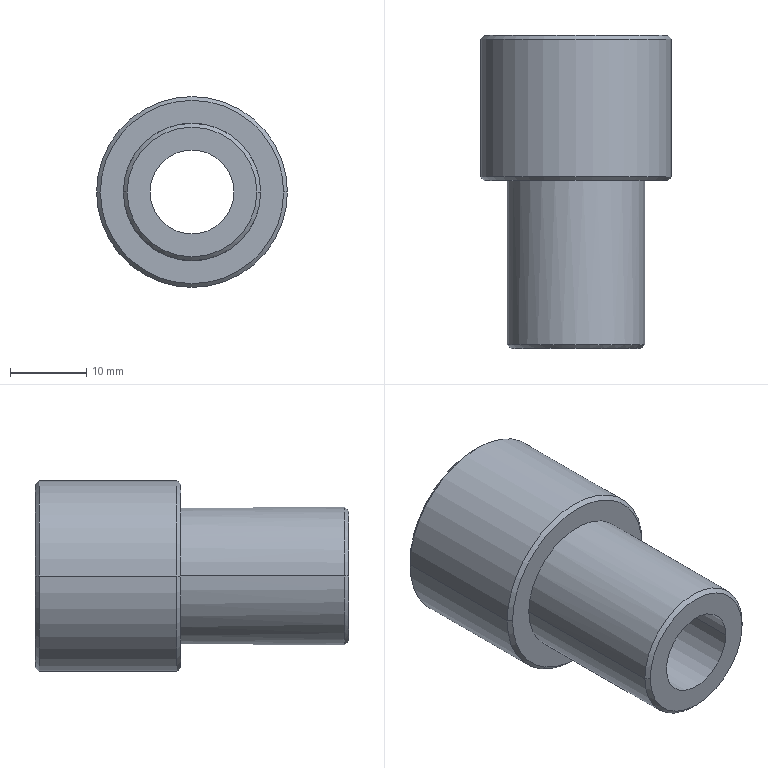Part | Creo | 1 solid | 20 faces | box 25 x 41 x 25 mm | volume 8763 mm3 | cylinder 8 | cone 8 | plane 4 | commonest cylinder face diameters 18 x4 11 x2 25 x2
STEP:
#1=CARTESIAN_POINT('',(-17.576,325.995,-174.076));
#2=VERTEX_POINT('',#1);
#3=CARTESIAN_POINT('',(-17.576,352.995,-174.076));
#4=VERTEX_POINT('',#3);
#5=CARTESIAN_POINT('',(-17.576,325.995,-174.076));
#6=DIRECTION('',(0.,1.,0.));
#7=VECTOR('',#6,27.);
#8=LINE('',#5,#7);
#9=EDGE_CURVE('',#2,#4,#8,.T.);
#10=ORIENTED_EDGE('',*,*,#9,.F.);
#11=CARTESIAN_POINT('',(-28.576,325.995,-174.076));
#12=VERTEX_POINT('',#11);
#13=CARTESIAN_POINT('',(-23.076,325.995,-174.076));
#14=DIRECTION('',(0.,1.,0.));
#15=DIRECTION('',(1.,0.,0.));
#16=AXIS2_PLACEMENT_3D('',#13,#14,#15);
#17=CIRCLE('',#16,5.5);
#18=EDGE_CURVE('',#2,#12,#17,.T.);
#19=ORIENTED_EDGE('',*,*,#18,.T.);
#20=CARTESIAN_POINT('',(-28.576,352.995,-174.076));
#21=VERTEX_POINT('',#20);
#22=CARTESIAN_POINT('',(-28.576,352.995,-174.076));
#23=DIRECTION('',(0.,-1.,0.));
#24=VECTOR('',#23,27.);
#25=LINE('',#22,#24);
#26=EDGE_CURVE('',#21,#12,#25,.T.);
#27=ORIENTED_EDGE('',*,*,#26,.F.);
#28=CARTESIAN_POINT('',(-23.076,352.995,-174.076));
#29=DIRECTION('',(0.,-1.,0.));
#30=DIRECTION('',(-1.,0.,0.));
#31=AXIS2_PLACEMENT_3D('',#28,#29,#30);
#32=CIRCLE('',#31,5.5);
#33=EDGE_CURVE('',#21,#4,#32,.T.);
#34=ORIENTED_EDGE('',*,*,#33,.T.);
#35=EDGE_LOOP('',(#10,#19,#27,#34));
#36=FACE_OUTER_BOUND('',#35,.F.);
#37=CARTESIAN_POINT('',(-23.076,343.995,-174.076));
#38=DIRECTION('',(0.,1.,0.));
#39=DIRECTION('',(-1.,0.,0.));
#40=AXIS2_PLACEMENT_3D('',#37,#38,#39);
#41=CYLINDRICAL_SURFACE('',#40,5.5);
#42=ADVANCED_FACE('',(#36),#41,.F.);
#43=ORIENTED_EDGE('',*,*,#26,.T.);
#44=CARTESIAN_POINT('',(-23.076,325.995,-174.076));
#45=DIRECTION('',(0.,1.,0.));
#46=DIRECTION('',(-1.,0.,0.));
#47=AXIS2_PLACEMENT_3D('',#44,#45,#46);
#48=CIRCLE('',#47,5.5);
#49=EDGE_CURVE('',#12,#2,#48,.T.);
#50=ORIENTED_EDGE('',*,*,#49,.T.);
#51=ORIENTED_EDGE('',*,*,#9,.T.);
#52=CARTESIAN_POINT('',(-23.076,352.995,-174.076));
#53=DIRECTION('',(0.,-1.,0.));
#54=DIRECTION('',(1.,0.,0.));
#55=AXIS2_PLACEMENT_3D('',#52,#53,#54);
#56=CIRCLE('',#55,5.5);
#57=EDGE_CURVE('',#4,#21,#56,.T.);
#58=ORIENTED_EDGE('',*,*,#57,.T.);
#59=EDGE_LOOP('',(#43,#50,#51,#58));
#60=FACE_OUTER_BOUND('',#59,.F.);
#61=CARTESIAN_POINT('',(-23.076,343.995,-174.076));
#62=DIRECTION('',(0.,1.,0.));
#63=DIRECTION('',(-1.,0.,0.));
#64=AXIS2_PLACEMENT_3D('',#61,#62,#63);
#65=CYLINDRICAL_SURFACE('',#64,5.5);
#66=ADVANCED_FACE('',(#60),#65,.F.);
#67=CARTESIAN_POINT('',(-31.576,325.995,-174.076));
#68=VERTEX_POINT('',#67);
#69=CARTESIAN_POINT('',(-23.076,325.995,-182.576));
#70=VERTEX_POINT('',#69);
#71=CARTESIAN_POINT('',(-23.076,325.995,-174.076));
#72=DIRECTION('',(0.,-1.,0.));
#73=DIRECTION('',(-1.,0.,0.));
#74=AXIS2_PLACEMENT_3D('',#71,#72,#73);
#75=CIRCLE('',#74,8.5);
#76=EDGE_CURVE('',#68,#70,#75,.T.);
#77=ORIENTED_EDGE('',*,*,#76,.F.);
#78=CARTESIAN_POINT('',(-23.076,325.995,-165.576));
#79=VERTEX_POINT('',#78);
#80=CARTESIAN_POINT('',(-23.076,325.995,-174.076));
#81=DIRECTION('',(0.,-1.,0.));
#82=DIRECTION('',(0.,0.,1.));
#83=AXIS2_PLACEMENT_3D('',#80,#81,#82);
#84=CIRCLE('',#83,8.5);
#85=EDGE_CURVE('',#79,#68,#84,.T.);
#86=ORIENTED_EDGE('',*,*,#85,.F.);
#87=CARTESIAN_POINT('',(-14.576,325.995,-174.076));
#88=VERTEX_POINT('',#87);
#89=CARTESIAN_POINT('',(-23.076,325.995,-174.076));
#90=DIRECTION('',(0.,-1.,0.));
#91=DIRECTION('',(1.,0.,0.));
#92=AXIS2_PLACEMENT_3D('',#89,#90,#91);
#93=CIRCLE('',#92,8.5);
#94=EDGE_CURVE('',#88,#79,#93,.T.);
#95=ORIENTED_EDGE('',*,*,#94,.F.);
#96=CARTESIAN_POINT('',(-23.076,325.995,-174.076));
#97=DIRECTION('',(0.,-1.,0.));
#98=DIRECTION('',(0.,0.,-1.));
#99=AXIS2_PLACEMENT_3D('',#96,#97,#98);
#100=CIRCLE('',#99,8.5);
#101=EDGE_CURVE('',#70,#88,#100,.T.);
#102=ORIENTED_EDGE('',*,*,#101,.F.);
#103=EDGE_LOOP('',(#77,#86,#95,#102));
#104=FACE_OUTER_BOUND('',#103,.F.);
#105=ORIENTED_EDGE('',*,*,#18,.F.);
#106=ORIENTED_EDGE('',*,*,#49,.F.);
#107=EDGE_LOOP('',(#105,#106));
#108=FACE_BOUND('',#107,.F.);
#109=CARTESIAN_POINT('',(16.924,325.995,-304.076));
#110=DIRECTION('',(0.,-1.,0.));
#111=DIRECTION('',(-1.,0.,0.));
#112=AXIS2_PLACEMENT_3D('',#109,#110,#111);
#113=PLANE('',#112);
#114=ADVANCED_FACE('',(#104,#108),#113,.T.);
#115=CARTESIAN_POINT('',(-32.076,326.495,-174.076));
#116=VERTEX_POINT('',#115);
#117=CARTESIAN_POINT('',(-31.576,325.995,-174.076));
#118=DIRECTION('',(-0.7071,0.7071,-0.000000008));
#119=VECTOR('',#118,0.7071);
#120=LINE('',#117,#119);
#121=EDGE_CURVE('',#68,#116,#120,.T.);
#122=ORIENTED_EDGE('',*,*,#121,.F.);
#123=ORIENTED_EDGE('',*,*,#76,.T.);
#124=ORIENTED_EDGE('',*,*,#101,.T.);
#125=CARTESIAN_POINT('',(-14.076,326.495,-174.076));
#126=VERTEX_POINT('',#125);
#127=CARTESIAN_POINT('',(-14.076,326.495,-174.076));
#128=DIRECTION('',(-0.7071,-0.7071,-0.000000008));
#129=VECTOR('',#128,0.7071);
#130=LINE('',#127,#129);
#131=EDGE_CURVE('',#126,#88,#130,.T.);
#132=ORIENTED_EDGE('',*,*,#131,.F.);
#133=CARTESIAN_POINT('',(-23.076,326.495,-183.076));
#134=VERTEX_POINT('',#133);
#135=CARTESIAN_POINT('',(-23.076,326.495,-174.076));
#136=DIRECTION('',(0.,-1.,0.));
#137=DIRECTION('',(0.,0.,-1.));
#138=AXIS2_PLACEMENT_3D('',#135,#136,#137);
#139=CIRCLE('',#138,9.);
#140=EDGE_CURVE('',#134,#126,#139,.T.);
#141=ORIENTED_EDGE('',*,*,#140,.F.);
#142=CARTESIAN_POINT('',(-23.076,326.495,-174.076));
#143=DIRECTION('',(0.,-1.,0.));
#144=DIRECTION('',(-1.,0.,0.));
#145=AXIS2_PLACEMENT_3D('',#142,#143,#144);
#146=CIRCLE('',#145,9.);
#147=EDGE_CURVE('',#116,#134,#146,.T.);
#148=ORIENTED_EDGE('',*,*,#147,.F.);
#149=EDGE_LOOP('',(#122,#123,#124,#132,#141,#148));
#150=FACE_OUTER_BOUND('',#149,.F.);
#151=CARTESIAN_POINT('',(-23.076,326.245,-174.076));
#152=DIRECTION('',(0.,1.,0.));
#153=DIRECTION('',(0.,0.,1.));
#154=AXIS2_PLACEMENT_3D('',#151,#152,#153);
#155=CONICAL_SURFACE('',#154,8.75,45.);
#156=ADVANCED_FACE('',(#150),#155,.T.);
#157=ORIENTED_EDGE('',*,*,#131,.T.);
#158=ORIENTED_EDGE('',*,*,#94,.T.);
#159=ORIENTED_EDGE('',*,*,#85,.T.);
#160=ORIENTED_EDGE('',*,*,#121,.T.);
#161=CARTESIAN_POINT('',(-23.076,326.495,-165.076));
#162=VERTEX_POINT('',#161);
#163=CARTESIAN_POINT('',(-23.076,326.495,-174.076));
#164=DIRECTION('',(0.,-1.,0.));
#165=DIRECTION('',(0.,0.,1.));
#166=AXIS2_PLACEMENT_3D('',#163,#164,#165);
#167=CIRCLE('',#166,9.);
#168=EDGE_CURVE('',#162,#116,#167,.T.);
#169=ORIENTED_EDGE('',*,*,#168,.F.);
#170=CARTESIAN_POINT('',(-23.076,326.495,-174.076));
#171=DIRECTION('',(0.,-1.,0.));
#172=DIRECTION('',(1.,0.,0.));
#173=AXIS2_PLACEMENT_3D('',#170,#171,#172);
#174=CIRCLE('',#173,9.);
#175=EDGE_CURVE('',#126,#162,#174,.T.);
#176=ORIENTED_EDGE('',*,*,#175,.F.);
#177=EDGE_LOOP('',(#157,#158,#159,#160,#169,#176));
#178=FACE_OUTER_BOUND('',#177,.F.);
#179=CARTESIAN_POINT('',(-23.076,326.245,-174.076));
#180=DIRECTION('',(0.,1.,0.));
#181=DIRECTION('',(0.,0.,1.));
#182=AXIS2_PLACEMENT_3D('',#179,#180,#181);
#183=CONICAL_SURFACE('',#182,8.75,45.);
#184=ADVANCED_FACE('',(#178),#183,.T.);
#185=CARTESIAN_POINT('',(-14.076,347.995,-174.076));
#186=VERTEX_POINT('',#185);
#187=CARTESIAN_POINT('',(-14.076,326.495,-174.076));
#188=DIRECTION('',(0.,1.,0.000000001));
#189=VECTOR('',#188,21.5);
#190=LINE('',#187,#189);
#191=EDGE_CURVE('',#126,#186,#190,.T.);
#192=ORIENTED_EDGE('',*,*,#191,.F.);
#193=ORIENTED_EDGE('',*,*,#175,.T.);
#194=ORIENTED_EDGE('',*,*,#168,.T.);
#195=CARTESIAN_POINT('',(-32.076,347.995,-174.076));
#196=VERTEX_POINT('',#195);
#197=CARTESIAN_POINT('',(-32.076,347.995,-174.076));
#198=DIRECTION('',(0.,-1.,0.000000001));
#199=VECTOR('',#198,21.5);
#200=LINE('',#197,#199);
#201=EDGE_CURVE('',#196,#116,#200,.T.);
#202=ORIENTED_EDGE('',*,*,#201,.F.);
#203=CARTESIAN_POINT('',(-23.076,347.995,-174.076));
#204=DIRECTION('',(0.,1.,0.));
#205=DIRECTION('',(-1.,0.,0.));
#206=AXIS2_PLACEMENT_3D('',#203,#204,#205);
#207=CIRCLE('',#206,9.);
#208=EDGE_CURVE('',#196,#186,#207,.T.);
#209=ORIENTED_EDGE('',*,*,#208,.T.);
#210=EDGE_LOOP('',(#192,#193,#194,#202,#209));
#211=FACE_OUTER_BOUND('',#210,.F.);
#212=CARTESIAN_POINT('',(-23.076,319.995,-174.076));
#213=DIRECTION('',(0.,-1.,0.));
#214=DIRECTION('',(-1.,0.,0.));
#215=AXIS2_PLACEMENT_3D('',#212,#213,#214);
#216=CYLINDRICAL_SURFACE('',#215,9.);
#217=ADVANCED_FACE('',(#211),#216,.T.);
#218=ORIENTED_EDGE('',*,*,#201,.T.);
#219=ORIENTED_EDGE('',*,*,#147,.T.);
#220=ORIENTED_EDGE('',*,*,#140,.T.);
#221=ORIENTED_EDGE('',*,*,#191,.T.);
#222=CARTESIAN_POINT('',(-23.076,347.995,-174.076));
#223=DIRECTION('',(0.,1.,0.));
#224=DIRECTION('',(1.,0.,0.));
#225=AXIS2_PLACEMENT_3D('',#222,#223,#224);
#226=CIRCLE('',#225,9.);
#227=EDGE_CURVE('',#186,#196,#226,.T.);
#228=ORIENTED_EDGE('',*,*,#227,.T.);
#229=EDGE_LOOP('',(#218,#219,#220,#221,#228));
#230=FACE_OUTER_BOUND('',#229,.F.);
#231=CARTESIAN_POINT('',(-23.076,319.995,-174.076));
#232=DIRECTION('',(0.,-1.,0.));
#233=DIRECTION('',(-1.,0.,0.));
#234=AXIS2_PLACEMENT_3D('',#231,#232,#233);
#235=CYLINDRICAL_SURFACE('',#234,9.);
#236=ADVANCED_FACE('',(#230),#235,.T.);
#237=CARTESIAN_POINT('',(-35.076,347.995,-174.076));
#238=VERTEX_POINT('',#237);
#239=CARTESIAN_POINT('',(-23.076,347.995,-186.076));
#240=VERTEX_POINT('',#239);
#241=CARTESIAN_POINT('',(-23.076,347.995,-174.076));
#242=DIRECTION('',(0.,-1.,0.));
#243=DIRECTION('',(-1.,0.,0.));
#244=AXIS2_PLACEMENT_3D('',#241,#242,#243);
#245=CIRCLE('',#244,12.);
#246=EDGE_CURVE('',#238,#240,#245,.T.);
#247=ORIENTED_EDGE('',*,*,#246,.F.);
#248=CARTESIAN_POINT('',(-23.076,347.995,-162.076));
#249=VERTEX_POINT('',#248);
#250=CARTESIAN_POINT('',(-23.076,347.995,-174.076));
#251=DIRECTION('',(0.,-1.,0.));
#252=DIRECTION('',(0.,0.,1.));
#253=AXIS2_PLACEMENT_3D('',#250,#251,#252);
#254=CIRCLE('',#253,12.);
#255=EDGE_CURVE('',#249,#238,#254,.T.);
#256=ORIENTED_EDGE('',*,*,#255,.F.);
#257=CARTESIAN_POINT('',(-11.076,347.995,-174.076));
#258=VERTEX_POINT('',#257);
#259=CARTESIAN_POINT('',(-23.076,347.995,-174.076));
#260=DIRECTION('',(0.,-1.,0.));
#261=DIRECTION('',(1.,0.,0.));
#262=AXIS2_PLACEMENT_3D('',#259,#260,#261);
#263=CIRCLE('',#262,12.);
#264=EDGE_CURVE('',#258,#249,#263,.T.);
#265=ORIENTED_EDGE('',*,*,#264,.F.);
#266=CARTESIAN_POINT('',(-23.076,347.995,-174.076));
#267=DIRECTION('',(0.,-1.,0.));
#268=DIRECTION('',(0.,0.,-1.));
#269=AXIS2_PLACEMENT_3D('',#266,#267,#268);
#270=CIRCLE('',#269,12.);
#271=EDGE_CURVE('',#240,#258,#270,.T.);
#272=ORIENTED_EDGE('',*,*,#271,.F.);
#273=EDGE_LOOP('',(#247,#256,#265,#272));
#274=FACE_OUTER_BOUND('',#273,.F.);
#275=ORIENTED_EDGE('',*,*,#227,.F.);
#276=ORIENTED_EDGE('',*,*,#208,.F.);
#277=EDGE_LOOP('',(#275,#276));
#278=FACE_BOUND('',#277,.F.);
#279=CARTESIAN_POINT('',(16.924,347.995,-304.076));
#280=DIRECTION('',(0.,-1.,0.));
#281=DIRECTION('',(-1.,0.,0.));
#282=AXIS2_PLACEMENT_3D('',#279,#280,#281);
#283=PLANE('',#282);
#284=ADVANCED_FACE('',(#274,#278),#283,.T.);
#285=CARTESIAN_POINT('',(-10.576,348.495,-174.076));
#286=VERTEX_POINT('',#285);
#287=CARTESIAN_POINT('',(-11.076,347.995,-174.076));
#288=DIRECTION('',(0.7071,0.7071,-0.000000007));
#289=VECTOR('',#288,0.7071);
#290=LINE('',#287,#289);
#291=EDGE_CURVE('',#258,#286,#290,.T.);
#292=ORIENTED_EDGE('',*,*,#291,.T.);
#293=CARTESIAN_POINT('',(-23.076,348.495,-186.576));
#294=VERTEX_POINT('',#293);
#295=CARTESIAN_POINT('',(-23.076,348.495,-174.076));
#296=DIRECTION('',(0.,-1.,0.));
#297=DIRECTION('',(0.,0.,-1.));
#298=AXIS2_PLACEMENT_3D('',#295,#296,#297);
#299=CIRCLE('',#298,12.5);
#300=EDGE_CURVE('',#294,#286,#299,.T.);
#301=ORIENTED_EDGE('',*,*,#300,.F.);
#302=CARTESIAN_POINT('',(-35.576,348.495,-174.076));
#303=VERTEX_POINT('',#302);
#304=CARTESIAN_POINT('',(-23.076,348.495,-174.076));
#305=DIRECTION('',(0.,-1.,0.));
#306=DIRECTION('',(-1.,0.,0.));
#307=AXIS2_PLACEMENT_3D('',#304,#305,#306);
#308=CIRCLE('',#307,12.5);
#309=EDGE_CURVE('',#303,#294,#308,.T.);
#310=ORIENTED_EDGE('',*,*,#309,.F.);
#311=CARTESIAN_POINT('',(-35.576,348.495,-174.076));
#312=DIRECTION('',(0.7071,-0.7071,-0.000000007));
#313=VECTOR('',#312,0.7071);
#314=LINE('',#311,#313);
#315=EDGE_CURVE('',#303,#238,#314,.T.);
#316=ORIENTED_EDGE('',*,*,#315,.T.);
#317=ORIENTED_EDGE('',*,*,#246,.T.);
#318=ORIENTED_EDGE('',*,*,#271,.T.);
#319=EDGE_LOOP('',(#292,#301,#310,#316,#317,#318));
#320=FACE_OUTER_BOUND('',#319,.F.);
#321=CARTESIAN_POINT('',(-23.076,348.245,-174.076));
#322=DIRECTION('',(0.,1.,0.));
#323=DIRECTION('',(0.,0.,1.));
#324=AXIS2_PLACEMENT_3D('',#321,#322,#323);
#325=CONICAL_SURFACE('',#324,12.25,45.);
#326=ADVANCED_FACE('',(#320),#325,.T.);
#327=ORIENTED_EDGE('',*,*,#315,.F.);
#328=CARTESIAN_POINT('',(-23.076,348.495,-161.576));
#329=VERTEX_POINT('',#328);
#330=CARTESIAN_POINT('',(-23.076,348.495,-174.076));
#331=DIRECTION('',(0.,-1.,0.));
#332=DIRECTION('',(0.,0.,1.));
#333=AXIS2_PLACEMENT_3D('',#330,#331,#332);
#334=CIRCLE('',#333,12.5);
#335=EDGE_CURVE('',#329,#303,#334,.T.);
#336=ORIENTED_EDGE('',*,*,#335,.F.);
#337=CARTESIAN_POINT('',(-23.076,348.495,-174.076));
#338=DIRECTION('',(0.,-1.,0.));
#339=DIRECTION('',(1.,0.,0.));
#340=AXIS2_PLACEMENT_3D('',#337,#338,#339);
#341=CIRCLE('',#340,12.5);
#342=EDGE_CURVE('',#286,#329,#341,.T.);
#343=ORIENTED_EDGE('',*,*,#342,.F.);
#344=ORIENTED_EDGE('',*,*,#291,.F.);
#345=ORIENTED_EDGE('',*,*,#264,.T.);
#346=ORIENTED_EDGE('',*,*,#255,.T.);
#347=EDGE_LOOP('',(#327,#336,#343,#344,#345,#346));
#348=FACE_OUTER_BOUND('',#347,.F.);
#349=CARTESIAN_POINT('',(-23.076,348.245,-174.076));
#350=DIRECTION('',(0.,1.,0.));
#351=DIRECTION('',(0.,0.,1.));
#352=AXIS2_PLACEMENT_3D('',#349,#350,#351);
#353=CONICAL_SURFACE('',#352,12.25,45.);
#354=ADVANCED_FACE('',(#348),#353,.T.);
#355=CARTESIAN_POINT('',(-35.576,366.495,-174.076));
#356=VERTEX_POINT('',#355);
#357=CARTESIAN_POINT('',(-35.576,366.495,-174.076));
#358=DIRECTION('',(0.,-1.,0.));
#359=VECTOR('',#358,18.);
#360=LINE('',#357,#359);
#361=EDGE_CURVE('',#356,#303,#360,.T.);
#362=ORIENTED_EDGE('',*,*,#361,.F.);
#363=CARTESIAN_POINT('',(-23.076,366.495,-161.576));
#364=VERTEX_POINT('',#363);
#365=CARTESIAN_POINT('',(-23.076,366.495,-174.076));
#366=DIRECTION('',(0.,1.,0.));
#367=DIRECTION('',(-1.,0.,0.));
#368=AXIS2_PLACEMENT_3D('',#365,#366,#367);
#369=CIRCLE('',#368,12.5);
#370=EDGE_CURVE('',#356,#364,#369,.T.);
#371=ORIENTED_EDGE('',*,*,#370,.T.);
#372=CARTESIAN_POINT('',(-10.576,366.495,-174.076));
#373=VERTEX_POINT('',#372);
#374=CARTESIAN_POINT('',(-23.076,366.495,-174.076));
#375=DIRECTION('',(0.,1.,0.));
#376=DIRECTION('',(0.,0.,1.));
#377=AXIS2_PLACEMENT_3D('',#374,#375,#376);
#378=CIRCLE('',#377,12.5);
#379=EDGE_CURVE('',#364,#373,#378,.T.);
#380=ORIENTED_EDGE('',*,*,#379,.T.);
#381=CARTESIAN_POINT('',(-10.576,348.495,-174.076));
#382=DIRECTION('',(0.,1.,0.));
#383=VECTOR('',#382,18.);
#384=LINE('',#381,#383);
#385=EDGE_CURVE('',#286,#373,#384,.T.);
#386=ORIENTED_EDGE('',*,*,#385,.F.);
#387=ORIENTED_EDGE('',*,*,#342,.T.);
#388=ORIENTED_EDGE('',*,*,#335,.T.);
#389=EDGE_LOOP('',(#362,#371,#380,#386,#387,#388));
#390=FACE_OUTER_BOUND('',#389,.F.);
#391=CARTESIAN_POINT('',(-23.076,328.995,-174.076));
#392=DIRECTION('',(0.,-1.,0.));
#393=DIRECTION('',(-1.,0.,0.));
#394=AXIS2_PLACEMENT_3D('',#391,#392,#393);
#395=CYLINDRICAL_SURFACE('',#394,12.5);
#396=ADVANCED_FACE('',(#390),#395,.T.);
#397=ORIENTED_EDGE('',*,*,#385,.T.);
#398=CARTESIAN_POINT('',(-23.076,366.495,-186.576));
#399=VERTEX_POINT('',#398);
#400=CARTESIAN_POINT('',(-23.076,366.495,-174.076));
#401=DIRECTION('',(0.,1.,0.));
#402=DIRECTION('',(1.,0.,0.));
#403=AXIS2_PLACEMENT_3D('',#400,#401,#402);
#404=CIRCLE('',#403,12.5);
#405=EDGE_CURVE('',#373,#399,#404,.T.);
#406=ORIENTED_EDGE('',*,*,#405,.T.);
#407=CARTESIAN_POINT('',(-23.076,366.495,-174.076));
#408=DIRECTION('',(0.,1.,0.));
#409=DIRECTION('',(0.,0.,-1.));
#410=AXIS2_PLACEMENT_3D('',#407,#408,#409);
#411=CIRCLE('',#410,12.5);
#412=EDGE_CURVE('',#399,#356,#411,.T.);
#413=ORIENTED_EDGE('',*,*,#412,.T.);
#414=ORIENTED_EDGE('',*,*,#361,.T.);
#415=ORIENTED_EDGE('',*,*,#309,.T.);
#416=ORIENTED_EDGE('',*,*,#300,.T.);
#417=EDGE_LOOP('',(#397,#406,#413,#414,#415,#416));
#418=FACE_OUTER_BOUND('',#417,.F.);
#419=CARTESIAN_POINT('',(-23.076,328.995,-174.076));
#420=DIRECTION('',(0.,-1.,0.));
#421=DIRECTION('',(-1.,0.,0.));
#422=AXIS2_PLACEMENT_3D('',#419,#420,#421);
#423=CYLINDRICAL_SURFACE('',#422,12.5);
#424=ADVANCED_FACE('',(#418),#423,.T.);
#425=CARTESIAN_POINT('',(-11.076,366.995,-174.076));
#426=VERTEX_POINT('',#425);
#427=CARTESIAN_POINT('',(-10.576,366.495,-174.076));
#428=DIRECTION('',(-0.7071,0.7071,0.000000011));
#429=VECTOR('',#428,0.7071);
#430=LINE('',#427,#429);
#431=EDGE_CURVE('',#373,#426,#430,.T.);
#432=ORIENTED_EDGE('',*,*,#431,.T.);
#433=CARTESIAN_POINT('',(-23.076,366.995,-186.076));
#434=VERTEX_POINT('',#433);
#435=CARTESIAN_POINT('',(-23.076,366.995,-174.076));
#436=DIRECTION('',(0.,1.,0.));
#437=DIRECTION('',(1.,0.,0.));
#438=AXIS2_PLACEMENT_3D('',#435,#436,#437);
#439=CIRCLE('',#438,12.);
#440=EDGE_CURVE('',#426,#434,#439,.T.);
#441=ORIENTED_EDGE('',*,*,#440,.T.);
#442=CARTESIAN_POINT('',(-35.076,366.995,-174.076));
#443=VERTEX_POINT('',#442);
#444=CARTESIAN_POINT('',(-23.076,366.995,-174.076));
#445=DIRECTION('',(0.,1.,0.));
#446=DIRECTION('',(0.,0.,-1.));
#447=AXIS2_PLACEMENT_3D('',#444,#445,#446);
#448=CIRCLE('',#447,12.);
#449=EDGE_CURVE('',#434,#443,#448,.T.);
#450=ORIENTED_EDGE('',*,*,#449,.T.);
#451=CARTESIAN_POINT('',(-35.076,366.995,-174.076));
#452=DIRECTION('',(-0.7071,-0.7071,0.000000011));
#453=VECTOR('',#452,0.7071);
#454=LINE('',#451,#453);
#455=EDGE_CURVE('',#443,#356,#454,.T.);
#456=ORIENTED_EDGE('',*,*,#455,.T.);
#457=ORIENTED_EDGE('',*,*,#412,.F.);
#458=ORIENTED_EDGE('',*,*,#405,.F.);
#459=EDGE_LOOP('',(#432,#441,#450,#456,#457,#458));
#460=FACE_OUTER_BOUND('',#459,.F.);
#461=CARTESIAN_POINT('',(-23.076,366.745,-174.076));
#462=DIRECTION('',(0.,-1.,0.));
#463=DIRECTION('',(0.,0.,1.));
#464=AXIS2_PLACEMENT_3D('',#461,#462,#463);
#465=CONICAL_SURFACE('',#464,12.25,45.);
#466=ADVANCED_FACE('',(#460),#465,.T.);
#467=ORIENTED_EDGE('',*,*,#455,.F.);
#468=CARTESIAN_POINT('',(-23.076,366.995,-162.076));
#469=VERTEX_POINT('',#468);
#470=CARTESIAN_POINT('',(-23.076,366.995,-174.076));
#471=DIRECTION('',(0.,1.,0.));
#472=DIRECTION('',(-1.,0.,0.));
#473=AXIS2_PLACEMENT_3D('',#470,#471,#472);
#474=CIRCLE('',#473,12.);
#475=EDGE_CURVE('',#443,#469,#474,.T.);
#476=ORIENTED_EDGE('',*,*,#475,.T.);
#477=CARTESIAN_POINT('',(-23.076,366.995,-174.076));
#478=DIRECTION('',(0.,1.,0.));
#479=DIRECTION('',(0.,0.,1.));
#480=AXIS2_PLACEMENT_3D('',#477,#478,#479);
#481=CIRCLE('',#480,12.);
#482=EDGE_CURVE('',#469,#426,#481,.T.);
#483=ORIENTED_EDGE('',*,*,#482,.T.);
#484=ORIENTED_EDGE('',*,*,#431,.F.);
#485=ORIENTED_EDGE('',*,*,#379,.F.);
#486=ORIENTED_EDGE('',*,*,#370,.F.);
#487=EDGE_LOOP('',(#467,#476,#483,#484,#485,#486));
#488=FACE_OUTER_BOUND('',#487,.F.);
#489=CARTESIAN_POINT('',(-23.076,366.745,-174.076));
#490=DIRECTION('',(0.,-1.,0.));
#491=DIRECTION('',(0.,0.,1.));
#492=AXIS2_PLACEMENT_3D('',#489,#490,#491);
#493=CONICAL_SURFACE('',#492,12.25,45.);
#494=ADVANCED_FACE('',(#488),#493,.T.);
#495=ORIENTED_EDGE('',*,*,#440,.F.);
#496=ORIENTED_EDGE('',*,*,#482,.F.);
#497=ORIENTED_EDGE('',*,*,#475,.F.);
#498=ORIENTED_EDGE('',*,*,#449,.F.);
#499=EDGE_LOOP('',(#495,#496,#497,#498));
#500=FACE_OUTER_BOUND('',#499,.F.);
#501=CARTESIAN_POINT('',(-32.576,366.995,-174.076));
#502=VERTEX_POINT('',#501);
#503=CARTESIAN_POINT('',(-23.076,366.995,-183.576));
#504=VERTEX_POINT('',#503);
#505=CARTESIAN_POINT('',(-23.076,366.995,-174.076));
#506=DIRECTION('',(0.,-1.,0.));
#507=DIRECTION('',(-1.,0.,0.));
#508=AXIS2_PLACEMENT_3D('',#505,#506,#507);
#509=CIRCLE('',#508,9.5);
#510=EDGE_CURVE('',#502,#504,#509,.T.);
#511=ORIENTED_EDGE('',*,*,#510,.F.);
#512=CARTESIAN_POINT('',(-23.076,366.995,-164.576));
#513=VERTEX_POINT('',#512);
#514=CARTESIAN_POINT('',(-23.076,366.995,-174.076));
#515=DIRECTION('',(0.,-1.,0.));
#516=DIRECTION('',(0.,0.,1.));
#517=AXIS2_PLACEMENT_3D('',#514,#515,#516);
#518=CIRCLE('',#517,9.5);
#519=EDGE_CURVE('',#513,#502,#518,.T.);
#520=ORIENTED_EDGE('',*,*,#519,.F.);
#521=CARTESIAN_POINT('',(-13.576,366.995,-174.076));
#522=VERTEX_POINT('',#521);
#523=CARTESIAN_POINT('',(-23.076,366.995,-174.076));
#524=DIRECTION('',(0.,-1.,0.));
#525=DIRECTION('',(1.,0.,0.));
#526=AXIS2_PLACEMENT_3D('',#523,#524,#525);
#527=CIRCLE('',#526,9.5);
#528=EDGE_CURVE('',#522,#513,#527,.T.);
#529=ORIENTED_EDGE('',*,*,#528,.F.);
#530=CARTESIAN_POINT('',(-23.076,366.995,-174.076));
#531=DIRECTION('',(0.,-1.,0.));
#532=DIRECTION('',(0.,0.,-1.));
#533=AXIS2_PLACEMENT_3D('',#530,#531,#532);
#534=CIRCLE('',#533,9.5);
#535=EDGE_CURVE('',#504,#522,#534,.T.);
#536=ORIENTED_EDGE('',*,*,#535,.F.);
#537=EDGE_LOOP('',(#511,#520,#529,#536));
#538=FACE_BOUND('',#537,.F.);
#539=CARTESIAN_POINT('',(16.924,366.995,-304.076));
#540=DIRECTION('',(0.,-1.,0.));
#541=DIRECTION('',(-1.,0.,0.));
#542=AXIS2_PLACEMENT_3D('',#539,#540,#541);
#543=PLANE('',#542);
#544=ADVANCED_FACE('',(#500,#538),#543,.F.);
#545=CARTESIAN_POINT('',(-32.076,366.495,-174.076));
#546=VERTEX_POINT('',#545);
#547=CARTESIAN_POINT('',(-32.576,366.995,-174.076));
#548=DIRECTION('',(0.7071,-0.7071,-0.000000021));
#549=VECTOR('',#548,0.7071);
#550=LINE('',#547,#549);
#551=EDGE_CURVE('',#502,#546,#550,.T.);
#552=ORIENTED_EDGE('',*,*,#551,.F.);
#553=ORIENTED_EDGE('',*,*,#510,.T.);
#554=ORIENTED_EDGE('',*,*,#535,.T.);
#555=CARTESIAN_POINT('',(-14.076,366.495,-174.076));
#556=VERTEX_POINT('',#555);
#557=CARTESIAN_POINT('',(-14.076,366.495,-174.076));
#558=DIRECTION('',(0.7071,0.7071,-0.000000021));
#559=VECTOR('',#558,0.7071);
#560=LINE('',#557,#559);
#561=EDGE_CURVE('',#556,#522,#560,.T.);
#562=ORIENTED_EDGE('',*,*,#561,.F.);
#563=CARTESIAN_POINT('',(-23.076,366.495,-183.076));
#564=VERTEX_POINT('',#563);
#565=CARTESIAN_POINT('',(-23.076,366.495,-174.076));
#566=DIRECTION('',(0.,-1.,0.));
#567=DIRECTION('',(0.,0.,-1.));
#568=AXIS2_PLACEMENT_3D('',#565,#566,#567);
#569=CIRCLE('',#568,9.);
#570=EDGE_CURVE('',#564,#556,#569,.T.);
#571=ORIENTED_EDGE('',*,*,#570,.F.);
#572=CARTESIAN_POINT('',(-23.076,366.495,-174.076));
#573=DIRECTION('',(0.,-1.,0.));
#574=DIRECTION('',(-1.,0.,0.));
#575=AXIS2_PLACEMENT_3D('',#572,#573,#574);
#576=CIRCLE('',#575,9.);
#577=EDGE_CURVE('',#546,#564,#576,.T.);
#578=ORIENTED_EDGE('',*,*,#577,.F.);
#579=EDGE_LOOP('',(#552,#553,#554,#562,#571,#578));
#580=FACE_OUTER_BOUND('',#579,.F.);
#581=CARTESIAN_POINT('',(-23.076,366.745,-174.076));
#582=DIRECTION('',(0.,1.,0.));
#583=DIRECTION('',(0.,0.,1.));
#584=AXIS2_PLACEMENT_3D('',#581,#582,#583);
#585=CONICAL_SURFACE('',#584,9.25,45.);
#586=ADVANCED_FACE('',(#580),#585,.F.);
#587=ORIENTED_EDGE('',*,*,#561,.T.);
#588=ORIENTED_EDGE('',*,*,#528,.T.);
#589=ORIENTED_EDGE('',*,*,#519,.T.);
#590=ORIENTED_EDGE('',*,*,#551,.T.);
#591=CARTESIAN_POINT('',(-23.076,366.495,-165.076));
#592=VERTEX_POINT('',#591);
#593=CARTESIAN_POINT('',(-23.076,366.495,-174.076));
#594=DIRECTION('',(0.,-1.,0.));
#595=DIRECTION('',(0.,0.,1.));
#596=AXIS2_PLACEMENT_3D('',#593,#594,#595);
#597=CIRCLE('',#596,9.);
#598=EDGE_CURVE('',#592,#546,#597,.T.);
#599=ORIENTED_EDGE('',*,*,#598,.F.);
#600=CARTESIAN_POINT('',(-23.076,366.495,-174.076));
#601=DIRECTION('',(0.,-1.,0.));
#602=DIRECTION('',(1.,0.,0.));
#603=AXIS2_PLACEMENT_3D('',#600,#601,#602);
#604=CIRCLE('',#603,9.);
#605=EDGE_CURVE('',#556,#592,#604,.T.);
#606=ORIENTED_EDGE('',*,*,#605,.F.);
#607=EDGE_LOOP('',(#587,#588,#589,#590,#599,#606));
#608=FACE_OUTER_BOUND('',#607,.F.);
#609=CARTESIAN_POINT('',(-23.076,366.745,-174.076));
#610=DIRECTION('',(0.,1.,0.));
#611=DIRECTION('',(0.,0.,1.));
#612=AXIS2_PLACEMENT_3D('',#609,#610,#611);
#613=CONICAL_SURFACE('',#612,9.25,45.);
#614=ADVANCED_FACE('',(#608),#613,.F.);
#615=CARTESIAN_POINT('',(-14.076,352.995,-174.076));
#616=VERTEX_POINT('',#615);
#617=CARTESIAN_POINT('',(-14.076,366.495,-174.076));
#618=DIRECTION('',(0.,-1.,0.000000003));
#619=VECTOR('',#618,13.5);
#620=LINE('',#617,#619);
#621=EDGE_CURVE('',#556,#616,#620,.T.);
#622=ORIENTED_EDGE('',*,*,#621,.F.);
#623=ORIENTED_EDGE('',*,*,#605,.T.);
#624=ORIENTED_EDGE('',*,*,#598,.T.);
#625=CARTESIAN_POINT('',(-32.076,352.995,-174.076));
#626=VERTEX_POINT('',#625);
#627=CARTESIAN_POINT('',(-32.076,352.995,-174.076));
#628=DIRECTION('',(0.,1.,0.000000003));
#629=VECTOR('',#628,13.5);
#630=LINE('',#627,#629);
#631=EDGE_CURVE('',#626,#546,#630,.T.);
#632=ORIENTED_EDGE('',*,*,#631,.F.);
#633=CARTESIAN_POINT('',(-23.076,352.995,-174.076));
#634=DIRECTION('',(0.,1.,0.));
#635=DIRECTION('',(-1.,0.,0.));
#636=AXIS2_PLACEMENT_3D('',#633,#634,#635);
#637=CIRCLE('',#636,9.);
#638=EDGE_CURVE('',#626,#616,#637,.T.);
#639=ORIENTED_EDGE('',*,*,#638,.T.);
#640=EDGE_LOOP('',(#622,#623,#624,#632,#639));
#641=FACE_OUTER_BOUND('',#640,.F.);
#642=CARTESIAN_POINT('',(-23.076,364.545,-174.076));
#643=DIRECTION('',(0.,-1.,0.));
#644=DIRECTION('',(-1.,0.,0.));
#645=AXIS2_PLACEMENT_3D('',#642,#643,#644);
#646=CYLINDRICAL_SURFACE('',#645,9.);
#647=ADVANCED_FACE('',(#641),#646,.F.);
#648=ORIENTED_EDGE('',*,*,#631,.T.);
#649=ORIENTED_EDGE('',*,*,#577,.T.);
#650=ORIENTED_EDGE('',*,*,#570,.T.);
#651=ORIENTED_EDGE('',*,*,#621,.T.);
#652=CARTESIAN_POINT('',(-23.076,352.995,-174.076));
#653=DIRECTION('',(0.,1.,0.));
#654=DIRECTION('',(1.,0.,0.));
#655=AXIS2_PLACEMENT_3D('',#652,#653,#654);
#656=CIRCLE('',#655,9.);
#657=EDGE_CURVE('',#616,#626,#656,.T.);
#658=ORIENTED_EDGE('',*,*,#657,.T.);
#659=EDGE_LOOP('',(#648,#649,#650,#651,#658));
#660=FACE_OUTER_BOUND('',#659,.F.);
#661=CARTESIAN_POINT('',(-23.076,364.545,-174.076));
#662=DIRECTION('',(0.,-1.,0.));
#663=DIRECTION('',(-1.,0.,0.));
#664=AXIS2_PLACEMENT_3D('',#661,#662,#663);
#665=CYLINDRICAL_SURFACE('',#664,9.);
#666=ADVANCED_FACE('',(#660),#665,.F.);
#667=ORIENTED_EDGE('',*,*,#657,.F.);
#668=ORIENTED_EDGE('',*,*,#638,.F.);
#669=EDGE_LOOP('',(#667,#668));
#670=FACE_OUTER_BOUND('',#669,.F.);
#671=ORIENTED_EDGE('',*,*,#33,.F.);
#672=ORIENTED_EDGE('',*,*,#57,.F.);
#673=EDGE_LOOP('',(#671,#672));
#674=FACE_BOUND('',#673,.F.);
#675=CARTESIAN_POINT('',(-23.076,352.995,-174.076));
#676=DIRECTION('',(0.,-1.,0.));
#677=DIRECTION('',(-1.,0.,0.));
#678=AXIS2_PLACEMENT_3D('',#675,#676,#677);
#679=PLANE('',#678);
#680=ADVANCED_FACE('',(#670,#674),#679,.F.);
#681=CLOSED_SHELL('',(#42,#66,#114,#156,#184,#217,#236,#284,#326,#354,#396,#424,#466,#494,#544,#586,#614,#647,#666,#680));
#682=MANIFOLD_SOLID_BREP('',#681);
#683=(LENGTH_UNIT()NAMED_UNIT(*)SI_UNIT(.MILLI.,.METRE.));
#684=UNCERTAINTY_MEASURE_WITH_UNIT(LENGTH_MEASURE(0.005414),#683,'','');
#685=(NAMED_UNIT(*)PLANE_ANGLE_UNIT()SI_UNIT($,.RADIAN.));
#686=PLANE_ANGLE_MEASURE_WITH_UNIT(PLANE_ANGLE_MEASURE(0.01745),#685);
#687=(CONVERSION_BASED_UNIT('DEGREE',#686)NAMED_UNIT(*)PLANE_ANGLE_UNIT());
#688=(NAMED_UNIT(*)SI_UNIT($,.STERADIAN.)SOLID_ANGLE_UNIT());
#689=(GEOMETRIC_REPRESENTATION_CONTEXT(3)GLOBAL_UNCERTAINTY_ASSIGNED_CONTEXT((#684))GLOBAL_UNIT_ASSIGNED_CONTEXT((#683,#687,#688))REPRESENTATION_CONTEXT('',''));
#690=ADVANCED_BREP_SHAPE_REPRESENTATION('',(#682),#689);